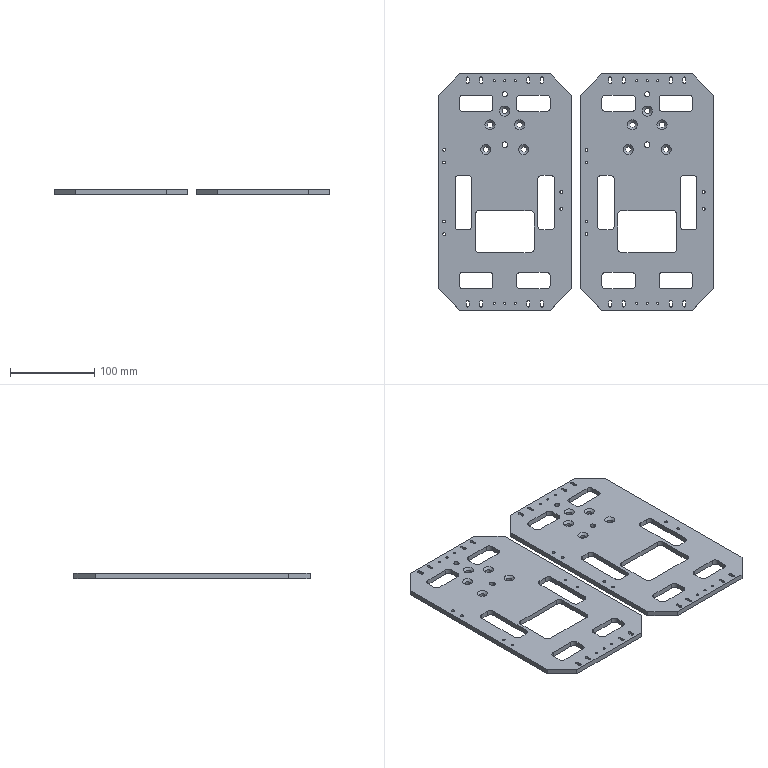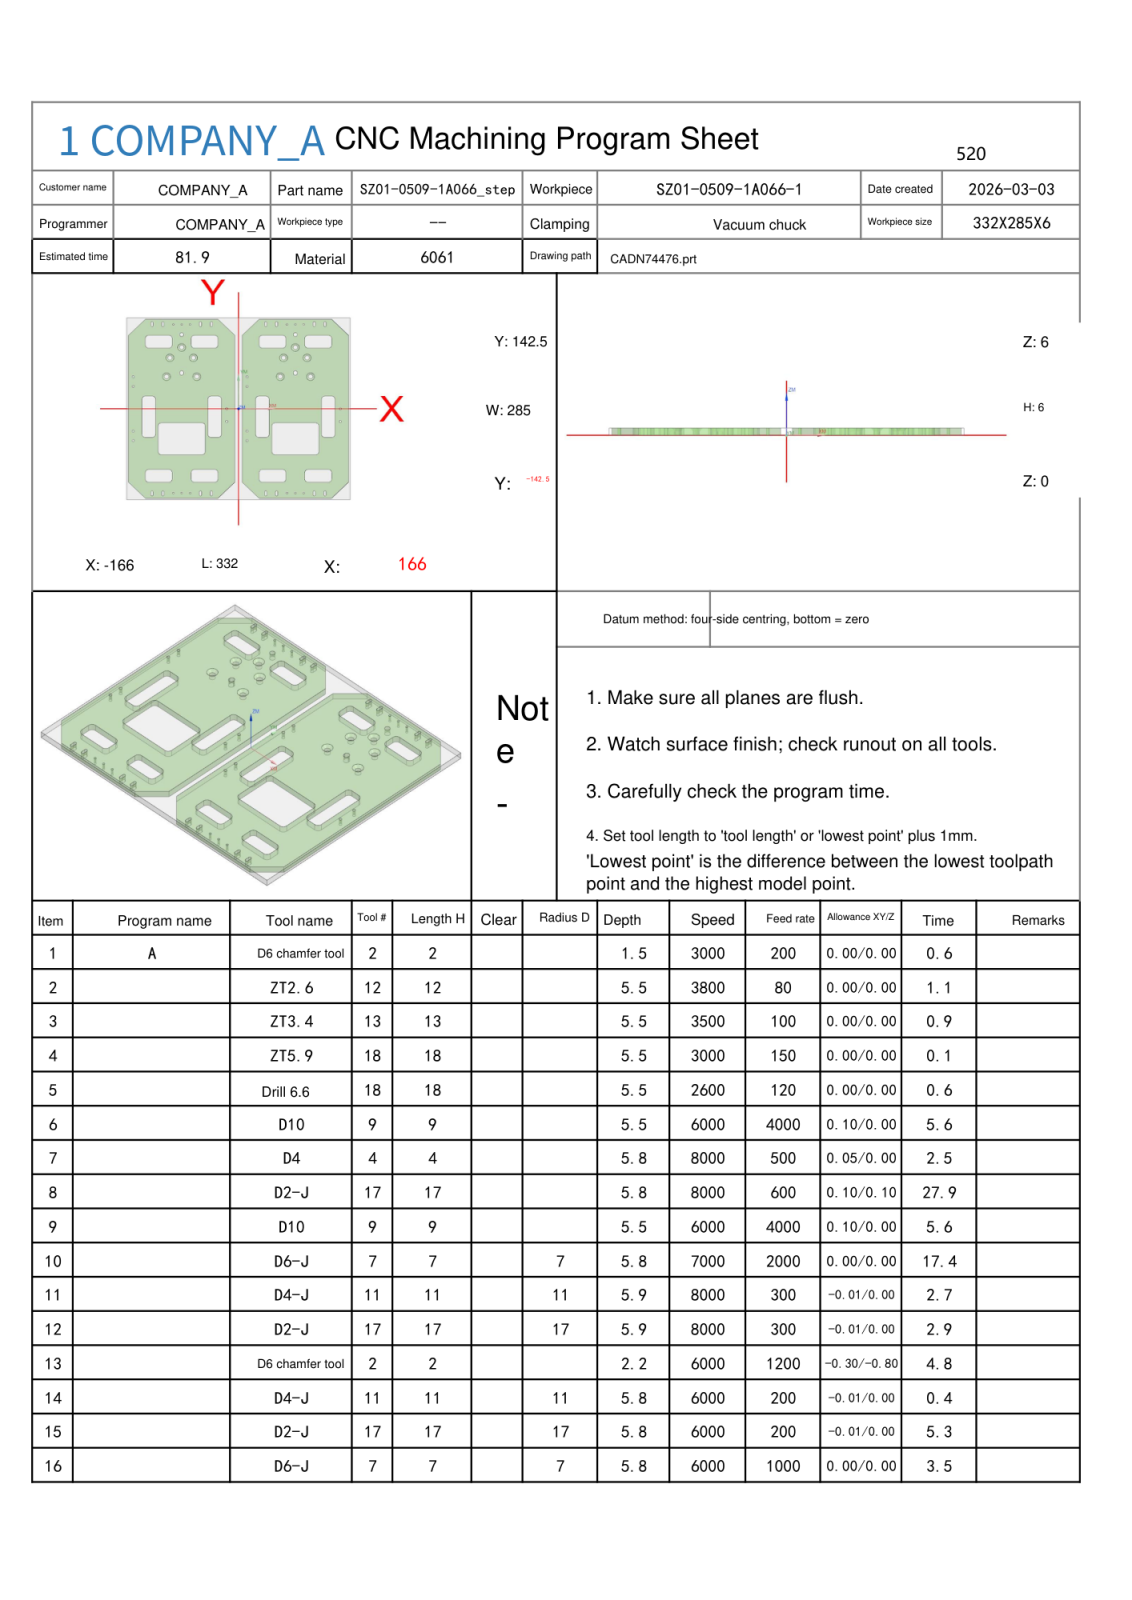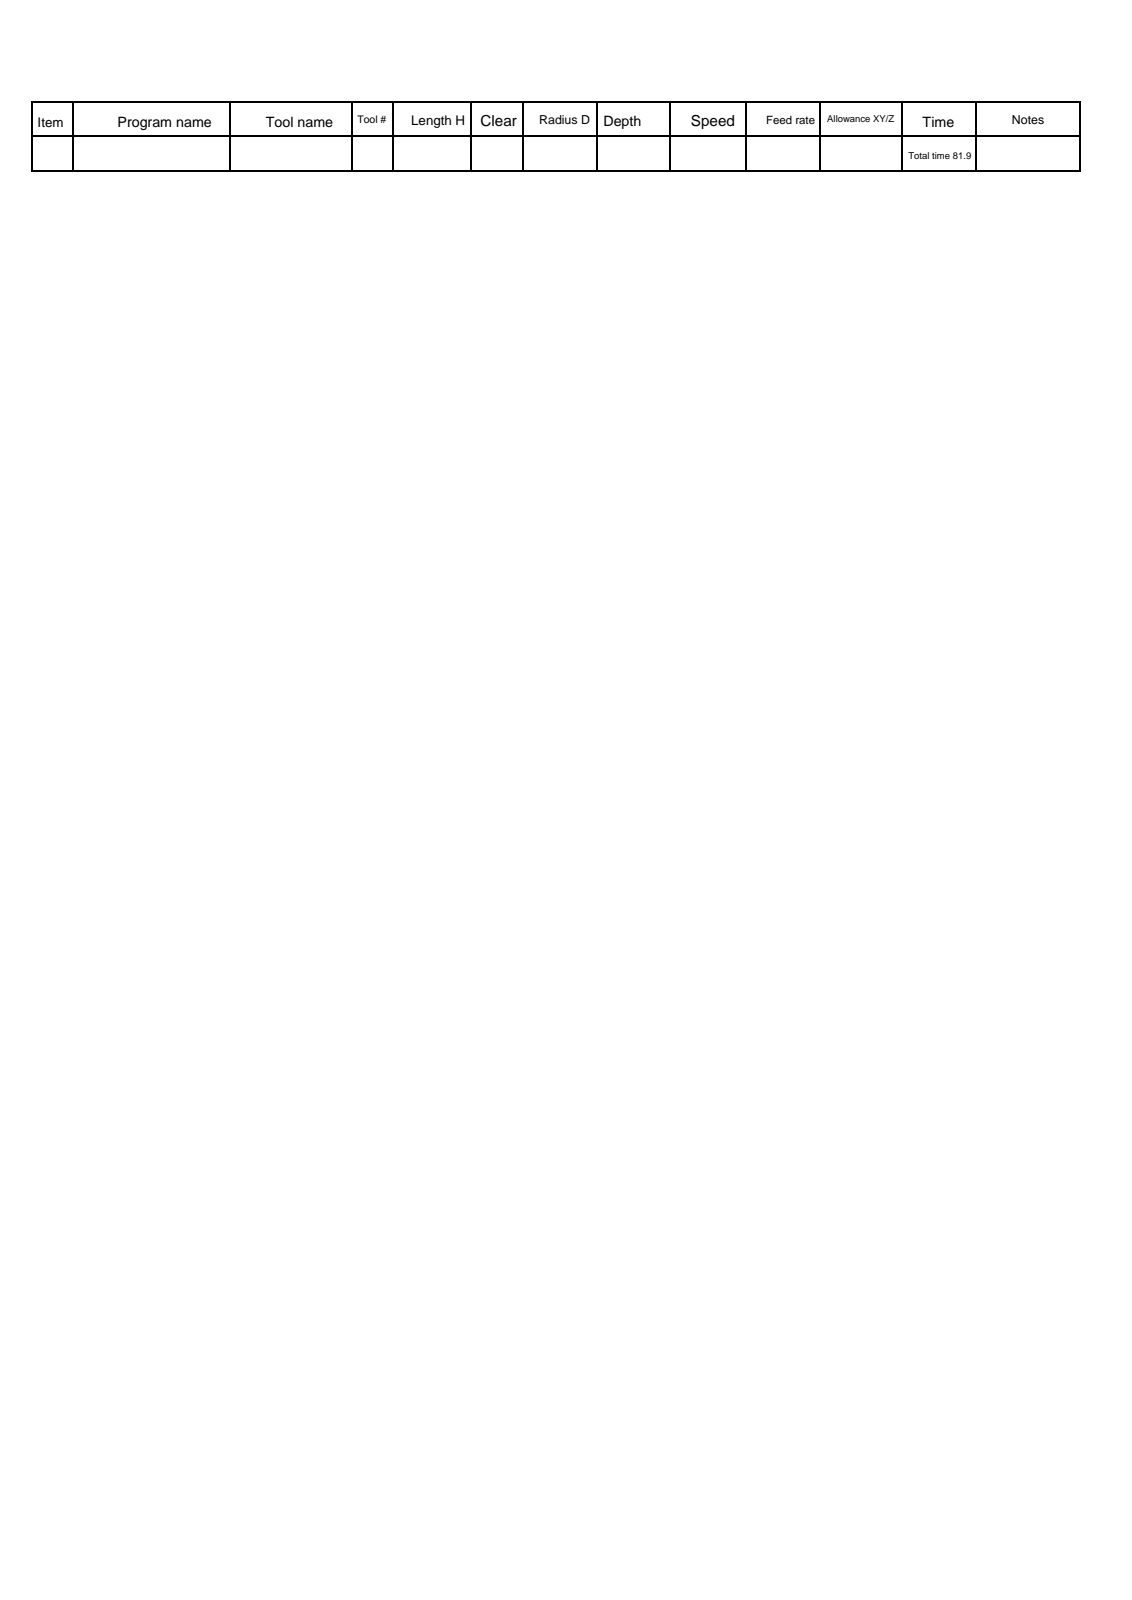NC program | NX | posted by the shop | part box 327 x 280 x 6 mm
Lines 9924 to 10362 of 31860:
N9 T09 M06
(D10  D=10. R=0. H=09 ce=0.10 di=0.00)
G00 G90 G54 X-168.6 Y0.0 M03 S6000
G43 H09 Z36.
M08
Z6.5
G01 Y115. Z6.432 F4000.
G02 X-167.106 Y118.606 Z6.43 I5.1 J0.0
G01 X-142.106 Y143.606 Z6.409
G02 X-138.5 Y145.1 Z6.407 I3.606 J-3.606
G01 X-30.5 Z6.343
G02 X-26.894 Y143.606 Z6.341 I0.0 J-5.1
G01 X-1.894 Y118.606 Z6.32
G02 X-.4 Y115. Z6.318 I-3.606 J-3.606
G01 Y-115. Z6.182
G02 X-1.894 Y-118.606 Z6.18 I-5.1 J0.0
G01 X-26.894 Y-143.606 Z6.159
G02 X-30.5 Y-145.1 Z6.157 I-3.606 J3.606
G01 X-138.5 Z6.093
G02 X-142.106 Y-143.606 Z6.091 I0.0 J5.1
G01 X-167.106 Y-118.606 Z6.07
G02 X-168.6 Y-115. Z6.068 I3.606 J3.606
G01 Y115. Z5.932
G02 X-167.106 Y118.606 Z5.93 I5.1 J0.0
G01 X-142.106 Y143.606 Z5.909
G02 X-138.5 Y145.1 Z5.907 I3.606 J-3.606
G01 X-30.5 Z5.843
G02 X-26.894 Y143.606 Z5.841 I0.0 J-5.1
G01 X-1.894 Y118.606 Z5.82
G02 X-.4 Y115. Z5.818 I-3.606 J-3.606
G01 Y-115. Z5.682
G02 X-1.894 Y-118.606 Z5.68 I-5.1 J0.0
G01 X-26.894 Y-143.606 Z5.659
G02 X-30.5 Y-145.1 Z5.657 I-3.606 J3.606
G01 X-138.5 Z5.593
G02 X-142.106 Y-143.606 Z5.591 I0.0 J5.1
G01 X-167.106 Y-118.606 Z5.57
G02 X-168.6 Y-115. Z5.568 I3.606 J3.606
G01 Y115. Z5.432
G02 X-167.106 Y118.606 Z5.43 I5.1 J0.0
G01 X-142.106 Y143.606 Z5.409
G02 X-138.5 Y145.1 Z5.407 I3.606 J-3.606
G01 X-30.5 Z5.343
G02 X-26.894 Y143.606 Z5.341 I0.0 J-5.1
G01 X-1.894 Y118.606 Z5.32
G02 X-.4 Y115. Z5.318 I-3.606 J-3.606
G01 Y-115. Z5.182
G02 X-1.894 Y-118.606 Z5.18 I-5.1 J0.0
G01 X-26.894 Y-143.606 Z5.159
G02 X-30.5 Y-145.1 Z5.157 I-3.606 J3.606
G01 X-138.5 Z5.093
G02 X-142.106 Y-143.606 Z5.091 I0.0 J5.1
G01 X-167.106 Y-118.606 Z5.07
G02 X-168.6 Y-115. Z5.068 I3.606 J3.606
G01 Y115. Z4.932
G02 X-167.106 Y118.606 Z4.93 I5.1 J0.0
G01 X-142.106 Y143.606 Z4.909
G02 X-138.5 Y145.1 Z4.907 I3.606 J-3.606
G01 X-30.5 Z4.843
G02 X-26.894 Y143.606 Z4.841 I0.0 J-5.1
G01 X-1.894 Y118.606 Z4.82
G02 X-.4 Y115. Z4.818 I-3.606 J-3.606
G01 Y-115. Z4.682
G02 X-1.894 Y-118.606 Z4.68 I-5.1 J0.0
G01 X-26.894 Y-143.606 Z4.659
G02 X-30.5 Y-145.1 Z4.657 I-3.606 J3.606
G01 X-138.5 Z4.593
G02 X-142.106 Y-143.606 Z4.591 I0.0 J5.1
G01 X-167.106 Y-118.606 Z4.57
G02 X-168.6 Y-115. Z4.568 I3.606 J3.606
G01 Y115. Z4.432
G02 X-167.106 Y118.606 Z4.43 I5.1 J0.0
G01 X-142.106 Y143.606 Z4.409
G02 X-138.5 Y145.1 Z4.407 I3.606 J-3.606
G01 X-30.5 Z4.343
G02 X-26.894 Y143.606 Z4.341 I0.0 J-5.1
G01 X-1.894 Y118.606 Z4.32
G02 X-.4 Y115. Z4.318 I-3.606 J-3.606
G01 Y-115. Z4.182
G02 X-1.894 Y-118.606 Z4.18 I-5.1 J0.0
G01 X-26.894 Y-143.606 Z4.159
G02 X-30.5 Y-145.1 Z4.157 I-3.606 J3.606
G01 X-138.5 Z4.093
G02 X-142.106 Y-143.606 Z4.091 I0.0 J5.1
G01 X-167.106 Y-118.606 Z4.07
G02 X-168.6 Y-115. Z4.068 I3.606 J3.606
G01 Y115. Z3.932
G02 X-167.106 Y118.606 Z3.93 I5.1 J0.0
G01 X-142.106 Y143.606 Z3.909
G02 X-138.5 Y145.1 Z3.907 I3.606 J-3.606
G01 X-30.5 Z3.843
G02 X-26.894 Y143.606 Z3.841 I0.0 J-5.1
G01 X-1.894 Y118.606 Z3.82
G02 X-.4 Y115. Z3.818 I-3.606 J-3.606
G01 Y-115. Z3.682
G02 X-1.894 Y-118.606 Z3.68 I-5.1 J0.0
G01 X-26.894 Y-143.606 Z3.659
G02 X-30.5 Y-145.1 Z3.657 I-3.606 J3.606
G01 X-138.5 Z3.593
G02 X-142.106 Y-143.606 Z3.591 I0.0 J5.1
G01 X-167.106 Y-118.606 Z3.57
G02 X-168.6 Y-115. Z3.568 I3.606 J3.606
G01 Y115. Z3.432
G02 X-167.106 Y118.606 Z3.43 I5.1 J0.0
G01 X-142.106 Y143.606 Z3.409
G02 X-138.5 Y145.1 Z3.407 I3.606 J-3.606
G01 X-30.5 Z3.343
G02 X-26.894 Y143.606 Z3.341 I0.0 J-5.1
G01 X-1.894 Y118.606 Z3.32
G02 X-.4 Y115. Z3.318 I-3.606 J-3.606
G01 Y-115. Z3.182
G02 X-1.894 Y-118.606 Z3.18 I-5.1 J0.0
G01 X-26.894 Y-143.606 Z3.159
G02 X-30.5 Y-145.1 Z3.157 I-3.606 J3.606
G01 X-138.5 Z3.093
G02 X-142.106 Y-143.606 Z3.091 I0.0 J5.1
G01 X-167.106 Y-118.606 Z3.07
G02 X-168.6 Y-115. Z3.068 I3.606 J3.606
G01 Y115. Z2.932
G02 X-167.106 Y118.606 Z2.93 I5.1 J0.0
G01 X-142.106 Y143.606 Z2.909
G02 X-138.5 Y145.1 Z2.907 I3.606 J-3.606
G01 X-30.5 Z2.843
G02 X-26.894 Y143.606 Z2.841 I0.0 J-5.1
G01 X-1.894 Y118.606 Z2.82
G02 X-.4 Y115. Z2.818 I-3.606 J-3.606
G01 Y-115. Z2.682
G02 X-1.894 Y-118.606 Z2.68 I-5.1 J0.0
G01 X-26.894 Y-143.606 Z2.659
G02 X-30.5 Y-145.1 Z2.657 I-3.606 J3.606
G01 X-138.5 Z2.593
G02 X-142.106 Y-143.606 Z2.591 I0.0 J5.1
G01 X-167.106 Y-118.606 Z2.57
G02 X-168.6 Y-115. Z2.568 I3.606 J3.606
G01 Y115. Z2.432
G02 X-167.106 Y118.606 Z2.43 I5.1 J0.0
G01 X-142.106 Y143.606 Z2.409
G02 X-138.5 Y145.1 Z2.407 I3.606 J-3.606
G01 X-30.5 Z2.343
G02 X-26.894 Y143.606 Z2.341 I0.0 J-5.1
G01 X-1.894 Y118.606 Z2.32
G02 X-.4 Y115. Z2.318 I-3.606 J-3.606
G01 Y-115. Z2.182
G02 X-1.894 Y-118.606 Z2.18 I-5.1 J0.0
G01 X-26.894 Y-143.606 Z2.159
G02 X-30.5 Y-145.1 Z2.157 I-3.606 J3.606
G01 X-138.5 Z2.093
G02 X-142.106 Y-143.606 Z2.091 I0.0 J5.1
G01 X-167.106 Y-118.606 Z2.07
G02 X-168.6 Y-115. Z2.068 I3.606 J3.606
G01 Y115. Z1.932
G02 X-167.106 Y118.606 Z1.93 I5.1 J0.0
G01 X-142.106 Y143.606 Z1.909
G02 X-138.5 Y145.1 Z1.907 I3.606 J-3.606
G01 X-30.5 Z1.843
G02 X-26.894 Y143.606 Z1.841 I0.0 J-5.1
G01 X-1.894 Y118.606 Z1.82
G02 X-.4 Y115. Z1.818 I-3.606 J-3.606
G01 Y-115. Z1.682
G02 X-1.894 Y-118.606 Z1.68 I-5.1 J0.0
G01 X-26.894 Y-143.606 Z1.659
G02 X-30.5 Y-145.1 Z1.657 I-3.606 J3.606
G01 X-138.5 Z1.593
G02 X-142.106 Y-143.606 Z1.591 I0.0 J5.1
G01 X-167.106 Y-118.606 Z1.57
G02 X-168.6 Y-115. Z1.568 I3.606 J3.606
G01 Y115. Z1.432
G02 X-167.106 Y118.606 Z1.43 I5.1 J0.0
G01 X-142.106 Y143.606 Z1.409
G02 X-138.5 Y145.1 Z1.407 I3.606 J-3.606
G01 X-30.5 Z1.343
G02 X-26.894 Y143.606 Z1.341 I0.0 J-5.1
G01 X-1.894 Y118.606 Z1.32
G02 X-.4 Y115. Z1.318 I-3.606 J-3.606
G01 Y-115. Z1.182
G02 X-1.894 Y-118.606 Z1.18 I-5.1 J0.0
G01 X-26.894 Y-143.606 Z1.159
G02 X-30.5 Y-145.1 Z1.157 I-3.606 J3.606
G01 X-138.5 Z1.093
G02 X-142.106 Y-143.606 Z1.091 I0.0 J5.1
G01 X-167.106 Y-118.606 Z1.07
G02 X-168.6 Y-115. Z1.068 I3.606 J3.606
G01 Y115. Z.932
G02 X-167.106 Y118.606 Z.93 I5.1 J0.0
G01 X-142.106 Y143.606 Z.909
G02 X-138.5 Y145.1 Z.907 I3.606 J-3.606
G01 X-30.5 Z.843
G02 X-26.894 Y143.606 Z.841 I0.0 J-5.1
G01 X-1.894 Y118.606 Z.82
G02 X-.4 Y115. Z.818 I-3.606 J-3.606
G01 Y-115. Z.682
G02 X-1.894 Y-118.606 Z.68 I-5.1 J0.0
G01 X-26.894 Y-143.606 Z.659
G02 X-30.5 Y-145.1 Z.657 I-3.606 J3.606
G01 X-138.5 Z.593
G02 X-142.106 Y-143.606 Z.591 I0.0 J5.1
G01 X-167.106 Y-118.606 Z.57
G02 X-168.6 Y-115. Z.568 I3.606 J3.606
G01 Y0.0 Z.5
Y115.
G02 X-167.106 Y118.606 I5.1 J0.0
G01 X-142.106 Y143.606
G02 X-138.5 Y145.1 I3.606 J-3.606
G01 X-30.5
G02 X-26.894 Y143.606 I0.0 J-5.1
G01 X-1.894 Y118.606
G02 X-.4 Y115. I-3.606 J-3.606
G01 Y-115.
G02 X-1.894 Y-118.606 I-5.1 J0.0
G01 X-26.894 Y-143.606
G02 X-30.5 Y-145.1 I-3.606 J3.606
G01 X-138.5
G02 X-142.106 Y-143.606 I0.0 J5.1
G01 X-167.106 Y-118.606
G02 X-168.6 Y-115. I3.606 J3.606
G01 Y0.0
Y.5
Z1.5
G00 Z36.
X168.6 Y0.0
Z6.5
G01 Y-115. Z6.432
G02 X167.106 Y-118.606 Z6.43 I-5.1 J0.0
G01 X142.106 Y-143.606 Z6.409
G02 X138.5 Y-145.1 Z6.407 I-3.606 J3.606
G01 X30.5 Z6.343
G02 X26.894 Y-143.606 Z6.341 I0.0 J5.1
G01 X1.894 Y-118.606 Z6.32
G02 X.4 Y-115. Z6.318 I3.606 J3.606
G01 Y115. Z6.182
G02 X1.894 Y118.606 Z6.18 I5.1 J0.0
G01 X26.894 Y143.606 Z6.159
G02 X30.5 Y145.1 Z6.157 I3.606 J-3.606
G01 X138.5 Z6.093
G02 X142.106 Y143.606 Z6.091 I0.0 J-5.1
G01 X167.106 Y118.606 Z6.07
G02 X168.6 Y115. Z6.068 I-3.606 J-3.606
G01 Y-115. Z5.932
G02 X167.106 Y-118.606 Z5.93 I-5.1 J0.0
G01 X142.106 Y-143.606 Z5.909
G02 X138.5 Y-145.1 Z5.907 I-3.606 J3.606
G01 X30.5 Z5.843
G02 X26.894 Y-143.606 Z5.841 I0.0 J5.1
G01 X1.894 Y-118.606 Z5.82
G02 X.4 Y-115. Z5.818 I3.606 J3.606
G01 Y115. Z5.682
G02 X1.894 Y118.606 Z5.68 I5.1 J0.0
G01 X26.894 Y143.606 Z5.659
G02 X30.5 Y145.1 Z5.657 I3.606 J-3.606
G01 X138.5 Z5.593
G02 X142.106 Y143.606 Z5.591 I0.0 J-5.1
G01 X167.106 Y118.606 Z5.57
G02 X168.6 Y115. Z5.568 I-3.606 J-3.606
G01 Y-115. Z5.432
G02 X167.106 Y-118.606 Z5.43 I-5.1 J0.0
G01 X142.106 Y-143.606 Z5.409
G02 X138.5 Y-145.1 Z5.407 I-3.606 J3.606
G01 X30.5 Z5.343
G02 X26.894 Y-143.606 Z5.341 I0.0 J5.1
G01 X1.894 Y-118.606 Z5.32
G02 X.4 Y-115. Z5.318 I3.606 J3.606
G01 Y115. Z5.182
G02 X1.894 Y118.606 Z5.18 I5.1 J0.0
G01 X26.894 Y143.606 Z5.159
G02 X30.5 Y145.1 Z5.157 I3.606 J-3.606
G01 X138.5 Z5.093
G02 X142.106 Y143.606 Z5.091 I0.0 J-5.1
G01 X167.106 Y118.606 Z5.07
G02 X168.6 Y115. Z5.068 I-3.606 J-3.606
G01 Y-115. Z4.932
G02 X167.106 Y-118.606 Z4.93 I-5.1 J0.0
G01 X142.106 Y-143.606 Z4.909
G02 X138.5 Y-145.1 Z4.907 I-3.606 J3.606
G01 X30.5 Z4.843
G02 X26.894 Y-143.606 Z4.841 I0.0 J5.1
G01 X1.894 Y-118.606 Z4.82
G02 X.4 Y-115. Z4.818 I3.606 J3.606
G01 Y115. Z4.682
G02 X1.894 Y118.606 Z4.68 I5.1 J0.0
G01 X26.894 Y143.606 Z4.659
G02 X30.5 Y145.1 Z4.657 I3.606 J-3.606
G01 X138.5 Z4.593
G02 X142.106 Y143.606 Z4.591 I0.0 J-5.1
G01 X167.106 Y118.606 Z4.57
G02 X168.6 Y115. Z4.568 I-3.606 J-3.606
G01 Y-115. Z4.432
G02 X167.106 Y-118.606 Z4.43 I-5.1 J0.0
G01 X142.106 Y-143.606 Z4.409
G02 X138.5 Y-145.1 Z4.407 I-3.606 J3.606
G01 X30.5 Z4.343
G02 X26.894 Y-143.606 Z4.341 I0.0 J5.1
G01 X1.894 Y-118.606 Z4.32
G02 X.4 Y-115. Z4.318 I3.606 J3.606
G01 Y115. Z4.182
G02 X1.894 Y118.606 Z4.18 I5.1 J0.0
G01 X26.894 Y143.606 Z4.159
G02 X30.5 Y145.1 Z4.157 I3.606 J-3.606
G01 X138.5 Z4.093
G02 X142.106 Y143.606 Z4.091 I0.0 J-5.1
G01 X167.106 Y118.606 Z4.07
G02 X168.6 Y115. Z4.068 I-3.606 J-3.606
G01 Y-115. Z3.932
G02 X167.106 Y-118.606 Z3.93 I-5.1 J0.0
G01 X142.106 Y-143.606 Z3.909
G02 X138.5 Y-145.1 Z3.907 I-3.606 J3.606
G01 X30.5 Z3.843
G02 X26.894 Y-143.606 Z3.841 I0.0 J5.1
G01 X1.894 Y-118.606 Z3.82
G02 X.4 Y-115. Z3.818 I3.606 J3.606
G01 Y115. Z3.682
G02 X1.894 Y118.606 Z3.68 I5.1 J0.0
G01 X26.894 Y143.606 Z3.659
G02 X30.5 Y145.1 Z3.657 I3.606 J-3.606
G01 X138.5 Z3.593
G02 X142.106 Y143.606 Z3.591 I0.0 J-5.1
G01 X167.106 Y118.606 Z3.57
G02 X168.6 Y115. Z3.568 I-3.606 J-3.606
G01 Y-115. Z3.432
G02 X167.106 Y-118.606 Z3.43 I-5.1 J0.0
G01 X142.106 Y-143.606 Z3.409
G02 X138.5 Y-145.1 Z3.407 I-3.606 J3.606
G01 X30.5 Z3.343
G02 X26.894 Y-143.606 Z3.341 I0.0 J5.1
G01 X1.894 Y-118.606 Z3.32
G02 X.4 Y-115. Z3.318 I3.606 J3.606
G01 Y115. Z3.182
G02 X1.894 Y118.606 Z3.18 I5.1 J0.0
G01 X26.894 Y143.606 Z3.159
G02 X30.5 Y145.1 Z3.157 I3.606 J-3.606
G01 X138.5 Z3.093
G02 X142.106 Y143.606 Z3.091 I0.0 J-5.1
G01 X167.106 Y118.606 Z3.07
G02 X168.6 Y115. Z3.068 I-3.606 J-3.606
G01 Y-115. Z2.932
G02 X167.106 Y-118.606 Z2.93 I-5.1 J0.0
G01 X142.106 Y-143.606 Z2.909
G02 X138.5 Y-145.1 Z2.907 I-3.606 J3.606
G01 X30.5 Z2.843
G02 X26.894 Y-143.606 Z2.841 I0.0 J5.1
G01 X1.894 Y-118.606 Z2.82
G02 X.4 Y-115. Z2.818 I3.606 J3.606
G01 Y115. Z2.682
G02 X1.894 Y118.606 Z2.68 I5.1 J0.0
G01 X26.894 Y143.606 Z2.659
G02 X30.5 Y145.1 Z2.657 I3.606 J-3.606
G01 X138.5 Z2.593
G02 X142.106 Y143.606 Z2.591 I0.0 J-5.1
G01 X167.106 Y118.606 Z2.57
G02 X168.6 Y115. Z2.568 I-3.606 J-3.606
G01 Y-115. Z2.432
G02 X167.106 Y-118.606 Z2.43 I-5.1 J0.0
G01 X142.106 Y-143.606 Z2.409
G02 X138.5 Y-145.1 Z2.407 I-3.606 J3.606
G01 X30.5 Z2.343
G02 X26.894 Y-143.606 Z2.341 I0.0 J5.1
G01 X1.894 Y-118.606 Z2.32
G02 X.4 Y-115. Z2.318 I3.606 J3.606
G01 Y115. Z2.182
G02 X1.894 Y118.606 Z2.18 I5.1 J0.0
G01 X26.894 Y143.606 Z2.159
G02 X30.5 Y145.1 Z2.157 I3.606 J-3.606
G01 X138.5 Z2.093
G02 X142.106 Y143.606 Z2.091 I0.0 J-5.1
G01 X167.106 Y118.606 Z2.07
G02 X168.6 Y115. Z2.068 I-3.606 J-3.606
G01 Y-115. Z1.932
G02 X167.106 Y-118.606 Z1.93 I-5.1 J0.0
G01 X142.106 Y-143.606 Z1.909
G02 X138.5 Y-145.1 Z1.907 I-3.606 J3.606
G01 X30.5 Z1.843
G02 X26.894 Y-143.606 Z1.841 I0.0 J5.1
G01 X1.894 Y-118.606 Z1.82
G02 X.4 Y-115. Z1.818 I3.606 J3.606
G01 Y115. Z1.682
G02 X1.894 Y118.606 Z1.68 I5.1 J0.0
G01 X26.894 Y143.606 Z1.659
G02 X30.5 Y145.1 Z1.657 I3.606 J-3.606
G01 X138.5 Z1.593
G02 X142.106 Y143.606 Z1.591 I0.0 J-5.1
G01 X167.106 Y118.606 Z1.57
G02 X168.6 Y115. Z1.568 I-3.606 J-3.606
G01 Y-115. Z1.432
G02 X167.106 Y-118.606 Z1.43 I-5.1 J0.0
G01 X142.106 Y-143.606 Z1.409
G02 X138.5 Y-145.1 Z1.407 I-3.606 J3.606
G01 X30.5 Z1.343
G02 X26.894 Y-143.606 Z1.341 I0.0 J5.1
G01 X1.894 Y-118.606 Z1.32
G02 X.4 Y-115. Z1.318 I3.606 J3.606
G01 Y115. Z1.182
G02 X1.894 Y118.606 Z1.18 I5.1 J0.0
G01 X26.894 Y143.606 Z1.159
G02 X30.5 Y145.1 Z1.157 I3.606 J-3.606
G01 X138.5 Z1.093
G02 X142.106 Y143.606 Z1.091 I0.0 J-5.1
G01 X167.106 Y118.606 Z1.07
G02 X168.6 Y115. Z1.068 I-3.606 J-3.606
G01 Y-115. Z.932
G02 X167.106 Y-118.606 Z.93 I-5.1 J0.0
G01 X142.106 Y-143.606 Z.909
G02 X138.5 Y-145.1 Z.907 I-3.606 J3.606
G01 X30.5 Z.843
G02 X26.894 Y-143.606 Z.841 I0.0 J5.1
G01 X1.894 Y-118.606 Z.82
G02 X.4 Y-115. Z.818 I3.606 J3.606
G01 Y115. Z.682
G02 X1.894 Y118.606 Z.68 I5.1 J0.0
G01 X26.894 Y143.606 Z.659
G02 X30.5 Y145.1 Z.657 I3.606 J-3.606
G01 X138.5 Z.593
G02 X142.106 Y143.606 Z.591 I0.0 J-5.1
G01 X167.106 Y118.606 Z.57
G02 X168.6 Y115. Z.568 I-3.606 J-3.606
G01 Y0.0 Z.5
Y-115.
G02 X167.106 Y-118.606 I-5.1 J0.0
G01 X142.106 Y-143.606
G02 X138.5 Y-145.1 I-3.606 J3.606
G01 X30.5
G02 X26.894 Y-143.606 I0.0 J5.1
G01 X1.894 Y-118.606
G02 X.4 Y-115. I3.606 J3.606
G01 Y115.
G02 X1.894 Y118.606 I5.1 J0.0
G01 X26.894 Y143.606
G02 X30.5 Y145.1 I3.606 J-3.606
G01 X138.5
G02 X142.106 Y143.606 I0.0 J-5.1
G01 X167.106 Y118.606
G02 X168.6 Y115. I-3.606 J-3.606
G01 Y0.0
Y-.5
Z1.5
G00 Z36.
G91 G28 Z0.0
M05
M09
G91 G28 Z0.0
M01